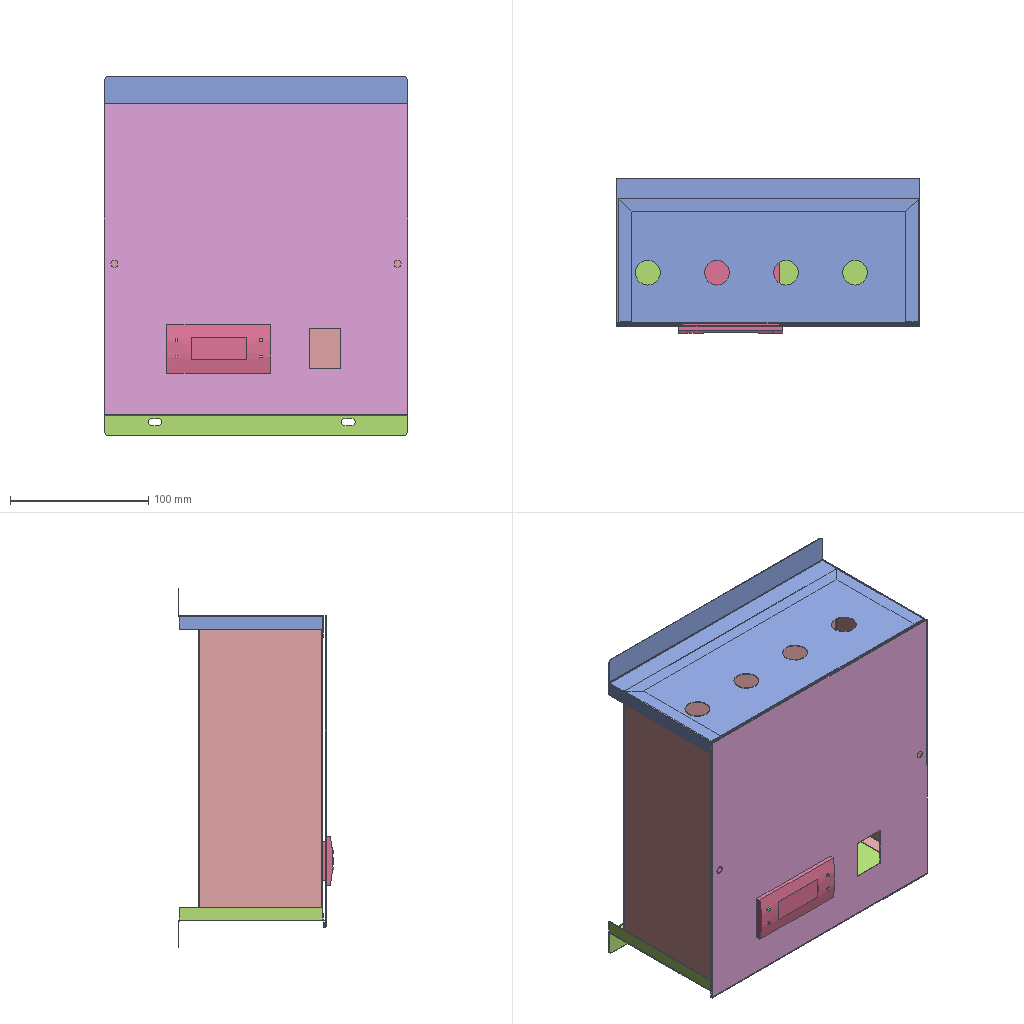Assembly | SolidWorks | 5 different items | 5 placed | box 220 x 113 x 261 mm
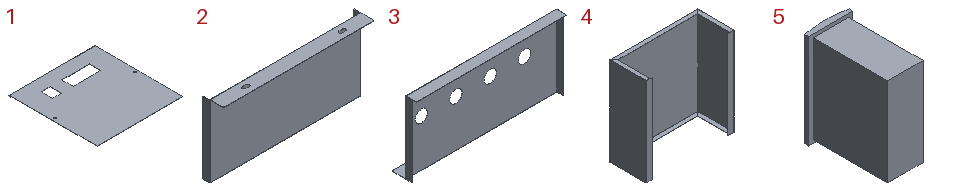Parts list (item | quantity | size | volume | features):
1 | x1 | 220 x 226 x 2 mm | 24067 mm3 | features 3DProfileFeature 1, FlatPattern 1, Hem 1, HoleWzd 1, ICE 1, SMBaseFlange 1, SheetMetal 1
2 | x1 | 220 x 29.5 x 105 mm | 15122 mm3 | features EdgeFlange 1, Fillet 1, FlatPattern 1, ICE 1, SMBaseFlange 1, SheetMetal 1
3 | x1 | 220 x 35.5 x 105 mm | 15806 mm3 | features EdgeFlange 1, Fillet 1, FlatPattern 1, ICE 1, SMBaseFlange 1, SheetMetal 1
4 | x1 | 218 x 90 x 220 mm | 50340 mm3 | features EdgeFlange 2, FlatPattern 1, SMBaseFlange 1, SheetMetal 1, UnFold 1
5 | x1 | 35 x 64.5 x 75 mm | 126879 mm3 | features Fillet 4, ICE 3, Extrusion 1
Mates (type | each side: item.copy, entity, surface, feature):
Coincident | 4.1 face plane Edge-Flange2 | 2.1 face plane Base-Flange1
Coincident | 4.1 face plane Edge-Flange1 | 2.1 face plane Edge-Flange1
Coincident | 4.1 face plane Edge-Flange2 | 2.1 face plane Edge-Flange1
Coincident | 4.1 face plane Edge-Flange2 | 3.1 face plane Edge-Flange1
Coincident | 4.1 face plane Edge-Flange1 | 3.1 face plane Edge-Flange1
Coincident | 4.1 face plane Edge-Flange2 | 3.1 face plane Base-Flange1
Coincident | 2.1 face plane Edge-Flange1 | 1.1 face plane Hem1
Parallel | 4.1 face plane Edge-Flange1 | 1.1 face plane Base-Flange1
Coincident | 2.1 face plane Edge-Flange1 | 1.1 face plane Base-Flange1
Coincident | 3.1 face plane Base-Flange1 | 1.1 face plane Base-Flange1
Coincident | 1.1 face plane Base-Flange1 | 5.1 face plane Boss-Extrude1
DistanceDim | 5.1 face plane Boss-Extrude3 | 1.1 face plane Extrude1 | 2 times